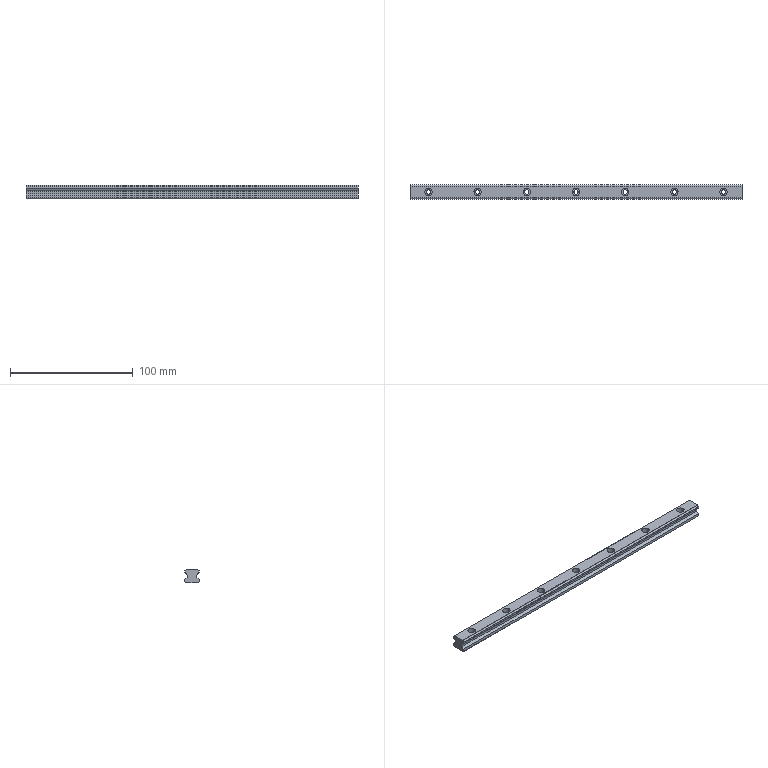Part | NX | 1 solid | 61 faces | box 270 x 12 x 11 mm | volume 28995 mm3 | cylinder 32 | plane 29 | commonest cylinder face diameters 3.5 x14 6 x14 2.5 x4